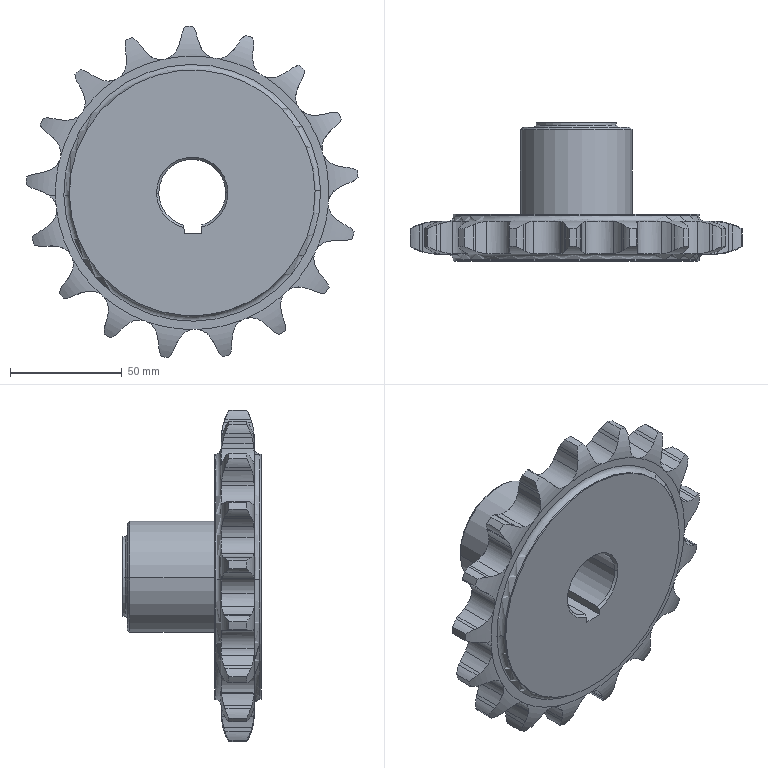Part | SolidWorks | features BaseBody 1 | 1 solid | 213 faces | box 148.61 x 61.823 x 148.247 mm | volume 292316 mm3 | cylinder 122 | plane 43 | torus 40 | cone 8 | commonest cylinder face diameters 23.3 x36 41.467 x35 16.059 x22 149 x17 110 x4 30 x3